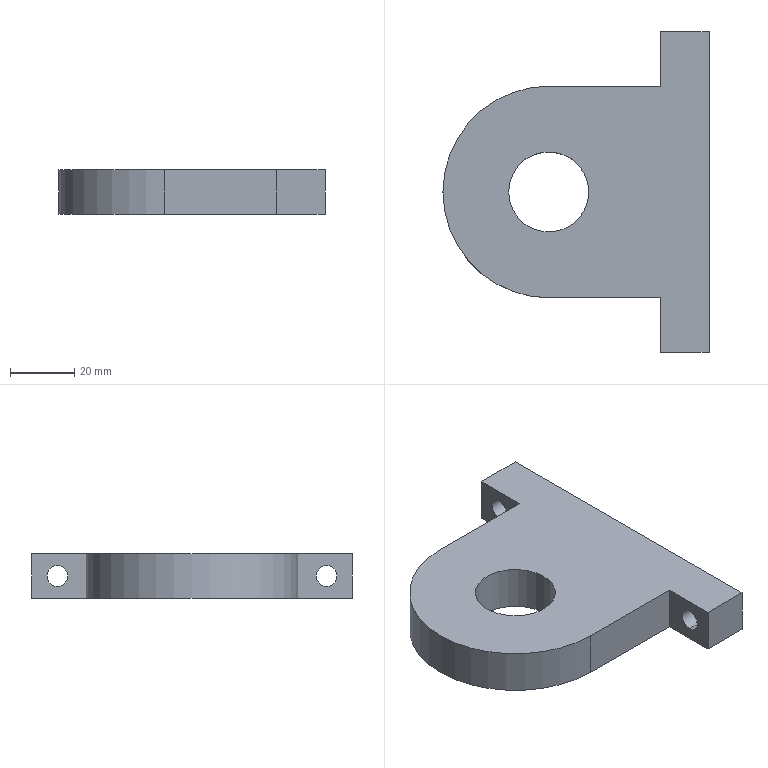Part | Creo | features DATUM PLANE 3, CURVE 2, COORDINATE SYSTEM 1, CUT 1, PROTRUSION 1 | 1 solid | 16 faces | box 83 x 100 x 14 mm | volume 69421 mm3 | plane 9 | cylinder 7 | commonest cylinder face diameters 6.5 x4 25 x2 66 x1
STEP:
#1=CARTESIAN_POINT('',(0.,0.,0.));
#2=DIRECTION('',(0.,0.,1.));
#3=DIRECTION('',(1.,0.,0.));
#4=AXIS2_PLACEMENT_3D('',#1,#2,#3);
#5=CARTESIAN_POINT('',(50.,50.,0.));
#6=VERTEX_POINT('',#5);
#7=CARTESIAN_POINT('',(35.,50.,0.));
#8=VERTEX_POINT('',#7);
#9=CARTESIAN_POINT('',(50.,50.,0.));
#10=DIRECTION('',(-1.,0.,0.));
#11=VECTOR('',#10,15.);
#12=LINE('',#9,#11);
#13=EDGE_CURVE('',#6,#8,#12,.T.);
#14=ORIENTED_EDGE('',*,*,#13,.T.);
#15=CARTESIAN_POINT('',(35.,33.,0.));
#16=VERTEX_POINT('',#15);
#17=CARTESIAN_POINT('',(35.,50.,0.));
#18=DIRECTION('',(0.,-1.,0.));
#19=VECTOR('',#18,17.);
#20=LINE('',#17,#19);
#21=EDGE_CURVE('',#8,#16,#20,.T.);
#22=ORIENTED_EDGE('',*,*,#21,.T.);
#23=CARTESIAN_POINT('',(0.,33.,0.));
#24=VERTEX_POINT('',#23);
#25=CARTESIAN_POINT('',(35.,33.,0.));
#26=DIRECTION('',(-1.,0.,0.));
#27=VECTOR('',#26,35.);
#28=LINE('',#25,#27);
#29=EDGE_CURVE('',#16,#24,#28,.T.);
#30=ORIENTED_EDGE('',*,*,#29,.T.);
#31=CARTESIAN_POINT('',(0.,-33.,0.));
#32=VERTEX_POINT('',#31);
#33=CARTESIAN_POINT('',(0.,0.,0.));
#34=DIRECTION('',(0.,0.,1.));
#35=DIRECTION('',(0.,1.,0.));
#36=AXIS2_PLACEMENT_3D('',#33,#34,#35);
#37=CIRCLE('',#36,33.);
#38=EDGE_CURVE('',#24,#32,#37,.T.);
#39=ORIENTED_EDGE('',*,*,#38,.T.);
#40=CARTESIAN_POINT('',(35.,-33.,0.));
#41=VERTEX_POINT('',#40);
#42=CARTESIAN_POINT('',(0.,-33.,0.));
#43=DIRECTION('',(1.,0.,0.));
#44=VECTOR('',#43,35.);
#45=LINE('',#42,#44);
#46=EDGE_CURVE('',#32,#41,#45,.T.);
#47=ORIENTED_EDGE('',*,*,#46,.T.);
#48=CARTESIAN_POINT('',(35.,-50.,0.));
#49=VERTEX_POINT('',#48);
#50=CARTESIAN_POINT('',(35.,-33.,0.));
#51=DIRECTION('',(0.,-1.,0.));
#52=VECTOR('',#51,17.);
#53=LINE('',#50,#52);
#54=EDGE_CURVE('',#41,#49,#53,.T.);
#55=ORIENTED_EDGE('',*,*,#54,.T.);
#56=CARTESIAN_POINT('',(50.,-50.,0.));
#57=VERTEX_POINT('',#56);
#58=CARTESIAN_POINT('',(35.,-50.,0.));
#59=DIRECTION('',(1.,0.,0.));
#60=VECTOR('',#59,15.);
#61=LINE('',#58,#60);
#62=EDGE_CURVE('',#49,#57,#61,.T.);
#63=ORIENTED_EDGE('',*,*,#62,.T.);
#64=CARTESIAN_POINT('',(50.,-50.,0.));
#65=DIRECTION('',(0.,1.,0.));
#66=VECTOR('',#65,100.);
#67=LINE('',#64,#66);
#68=EDGE_CURVE('',#57,#6,#67,.T.);
#69=ORIENTED_EDGE('',*,*,#68,.T.);
#70=EDGE_LOOP('',(#14,#22,#30,#39,#47,#55,#63,#69));
#71=FACE_OUTER_BOUND('',#70,.F.);
#72=CARTESIAN_POINT('',(12.5,0.,0.));
#73=VERTEX_POINT('',#72);
#74=CARTESIAN_POINT('',(-12.5,0.,0.));
#75=VERTEX_POINT('',#74);
#76=CARTESIAN_POINT('',(0.,0.,0.));
#77=DIRECTION('',(0.,0.,-1.));
#78=DIRECTION('',(1.,0.,0.));
#79=AXIS2_PLACEMENT_3D('',#76,#77,#78);
#80=CIRCLE('',#79,12.5);
#81=EDGE_CURVE('',#73,#75,#80,.T.);
#82=ORIENTED_EDGE('',*,*,#81,.T.);
#83=CARTESIAN_POINT('',(0.,0.,0.));
#84=DIRECTION('',(0.,0.,-1.));
#85=DIRECTION('',(-1.,0.,0.));
#86=AXIS2_PLACEMENT_3D('',#83,#84,#85);
#87=CIRCLE('',#86,12.5);
#88=EDGE_CURVE('',#75,#73,#87,.T.);
#89=ORIENTED_EDGE('',*,*,#88,.T.);
#90=EDGE_LOOP('',(#82,#89));
#91=FACE_BOUND('',#90,.F.);
#92=CARTESIAN_POINT('',(0.,0.,0.));
#93=DIRECTION('',(0.,0.,1.));
#94=DIRECTION('',(1.,0.,0.));
#95=AXIS2_PLACEMENT_3D('',#92,#93,#94);
#96=PLANE('',#95);
#97=ADVANCED_FACE('',(#71,#91),#96,.F.);
#98=ORIENTED_EDGE('',*,*,#81,.F.);
#99=CARTESIAN_POINT('',(12.5,0.,14.));
#100=VERTEX_POINT('',#99);
#101=CARTESIAN_POINT('',(12.5,0.,0.));
#102=DIRECTION('',(0.,0.,1.));
#103=VECTOR('',#102,14.);
#104=LINE('',#101,#103);
#105=EDGE_CURVE('',#73,#100,#104,.T.);
#106=ORIENTED_EDGE('',*,*,#105,.T.);
#107=CARTESIAN_POINT('',(-12.5,0.,14.));
#108=VERTEX_POINT('',#107);
#109=CARTESIAN_POINT('',(0.,0.,14.));
#110=DIRECTION('',(0.,0.,-1.));
#111=DIRECTION('',(1.,0.,0.));
#112=AXIS2_PLACEMENT_3D('',#109,#110,#111);
#113=CIRCLE('',#112,12.5);
#114=EDGE_CURVE('',#100,#108,#113,.T.);
#115=ORIENTED_EDGE('',*,*,#114,.T.);
#116=CARTESIAN_POINT('',(-12.5,0.,0.));
#117=DIRECTION('',(0.,0.,1.));
#118=VECTOR('',#117,14.);
#119=LINE('',#116,#118);
#120=EDGE_CURVE('',#75,#108,#119,.T.);
#121=ORIENTED_EDGE('',*,*,#120,.F.);
#122=EDGE_LOOP('',(#98,#106,#115,#121));
#123=FACE_OUTER_BOUND('',#122,.F.);
#124=CARTESIAN_POINT('',(0.,0.,0.));
#125=DIRECTION('',(0.,0.,1.));
#126=DIRECTION('',(1.,0.,0.));
#127=AXIS2_PLACEMENT_3D('',#124,#125,#126);
#128=CYLINDRICAL_SURFACE('',#127,12.5);
#129=ADVANCED_FACE('',(#123),#128,.F.);
#130=ORIENTED_EDGE('',*,*,#88,.F.);
#131=ORIENTED_EDGE('',*,*,#120,.T.);
#132=CARTESIAN_POINT('',(0.,0.,14.));
#133=DIRECTION('',(0.,0.,-1.));
#134=DIRECTION('',(-1.,0.,0.));
#135=AXIS2_PLACEMENT_3D('',#132,#133,#134);
#136=CIRCLE('',#135,12.5);
#137=EDGE_CURVE('',#108,#100,#136,.T.);
#138=ORIENTED_EDGE('',*,*,#137,.T.);
#139=ORIENTED_EDGE('',*,*,#105,.F.);
#140=EDGE_LOOP('',(#130,#131,#138,#139));
#141=FACE_OUTER_BOUND('',#140,.F.);
#142=CARTESIAN_POINT('',(0.,0.,0.));
#143=DIRECTION('',(0.,0.,1.));
#144=DIRECTION('',(1.,0.,0.));
#145=AXIS2_PLACEMENT_3D('',#142,#143,#144);
#146=CYLINDRICAL_SURFACE('',#145,12.5);
#147=ADVANCED_FACE('',(#141),#146,.F.);
#148=CARTESIAN_POINT('',(50.,50.,14.));
#149=VERTEX_POINT('',#148);
#150=CARTESIAN_POINT('',(35.,50.,14.));
#151=VERTEX_POINT('',#150);
#152=CARTESIAN_POINT('',(50.,50.,14.));
#153=DIRECTION('',(-1.,0.,0.));
#154=VECTOR('',#153,15.);
#155=LINE('',#152,#154);
#156=EDGE_CURVE('',#149,#151,#155,.T.);
#157=ORIENTED_EDGE('',*,*,#156,.F.);
#158=CARTESIAN_POINT('',(50.,-50.,14.));
#159=VERTEX_POINT('',#158);
#160=CARTESIAN_POINT('',(50.,-50.,14.));
#161=DIRECTION('',(0.,1.,0.));
#162=VECTOR('',#161,100.);
#163=LINE('',#160,#162);
#164=EDGE_CURVE('',#159,#149,#163,.T.);
#165=ORIENTED_EDGE('',*,*,#164,.F.);
#166=CARTESIAN_POINT('',(35.,-50.,14.));
#167=VERTEX_POINT('',#166);
#168=CARTESIAN_POINT('',(35.,-50.,14.));
#169=DIRECTION('',(1.,0.,0.));
#170=VECTOR('',#169,15.);
#171=LINE('',#168,#170);
#172=EDGE_CURVE('',#167,#159,#171,.T.);
#173=ORIENTED_EDGE('',*,*,#172,.F.);
#174=CARTESIAN_POINT('',(35.,-33.,14.));
#175=VERTEX_POINT('',#174);
#176=CARTESIAN_POINT('',(35.,-33.,14.));
#177=DIRECTION('',(0.,-1.,0.));
#178=VECTOR('',#177,17.);
#179=LINE('',#176,#178);
#180=EDGE_CURVE('',#175,#167,#179,.T.);
#181=ORIENTED_EDGE('',*,*,#180,.F.);
#182=CARTESIAN_POINT('',(0.,-33.,14.));
#183=VERTEX_POINT('',#182);
#184=CARTESIAN_POINT('',(0.,-33.,14.));
#185=DIRECTION('',(1.,0.,0.));
#186=VECTOR('',#185,35.);
#187=LINE('',#184,#186);
#188=EDGE_CURVE('',#183,#175,#187,.T.);
#189=ORIENTED_EDGE('',*,*,#188,.F.);
#190=CARTESIAN_POINT('',(0.,33.,14.));
#191=VERTEX_POINT('',#190);
#192=CARTESIAN_POINT('',(0.,0.,14.));
#193=DIRECTION('',(0.,0.,1.));
#194=DIRECTION('',(0.,1.,0.));
#195=AXIS2_PLACEMENT_3D('',#192,#193,#194);
#196=CIRCLE('',#195,33.);
#197=EDGE_CURVE('',#191,#183,#196,.T.);
#198=ORIENTED_EDGE('',*,*,#197,.F.);
#199=CARTESIAN_POINT('',(35.,33.,14.));
#200=VERTEX_POINT('',#199);
#201=CARTESIAN_POINT('',(35.,33.,14.));
#202=DIRECTION('',(-1.,0.,0.));
#203=VECTOR('',#202,35.);
#204=LINE('',#201,#203);
#205=EDGE_CURVE('',#200,#191,#204,.T.);
#206=ORIENTED_EDGE('',*,*,#205,.F.);
#207=CARTESIAN_POINT('',(35.,50.,14.));
#208=DIRECTION('',(0.,-1.,0.));
#209=VECTOR('',#208,17.);
#210=LINE('',#207,#209);
#211=EDGE_CURVE('',#151,#200,#210,.T.);
#212=ORIENTED_EDGE('',*,*,#211,.F.);
#213=EDGE_LOOP('',(#157,#165,#173,#181,#189,#198,#206,#212));
#214=FACE_OUTER_BOUND('',#213,.F.);
#215=ORIENTED_EDGE('',*,*,#114,.F.);
#216=ORIENTED_EDGE('',*,*,#137,.F.);
#217=EDGE_LOOP('',(#215,#216));
#218=FACE_BOUND('',#217,.F.);
#219=CARTESIAN_POINT('',(0.,0.,14.));
#220=DIRECTION('',(0.,0.,1.));
#221=DIRECTION('',(1.,0.,0.));
#222=AXIS2_PLACEMENT_3D('',#219,#220,#221);
#223=PLANE('',#222);
#224=ADVANCED_FACE('',(#214,#218),#223,.T.);
#225=ORIENTED_EDGE('',*,*,#13,.F.);
#226=CARTESIAN_POINT('',(50.,50.,0.));
#227=DIRECTION('',(0.,0.,1.));
#228=VECTOR('',#227,14.);
#229=LINE('',#226,#228);
#230=EDGE_CURVE('',#6,#149,#229,.T.);
#231=ORIENTED_EDGE('',*,*,#230,.T.);
#232=ORIENTED_EDGE('',*,*,#156,.T.);
#233=CARTESIAN_POINT('',(35.,50.,0.));
#234=DIRECTION('',(0.,0.,1.));
#235=VECTOR('',#234,14.);
#236=LINE('',#233,#235);
#237=EDGE_CURVE('',#8,#151,#236,.T.);
#238=ORIENTED_EDGE('',*,*,#237,.F.);
#239=EDGE_LOOP('',(#225,#231,#232,#238));
#240=FACE_OUTER_BOUND('',#239,.F.);
#241=CARTESIAN_POINT('',(50.,50.,0.));
#242=DIRECTION('',(0.,1.,0.));
#243=DIRECTION('',(-1.,0.,0.));
#244=AXIS2_PLACEMENT_3D('',#241,#242,#243);
#245=PLANE('',#244);
#246=ADVANCED_FACE('',(#240),#245,.T.);
#247=ORIENTED_EDGE('',*,*,#68,.F.);
#248=CARTESIAN_POINT('',(50.,-50.,0.));
#249=DIRECTION('',(0.,0.,1.));
#250=VECTOR('',#249,14.);
#251=LINE('',#248,#250);
#252=EDGE_CURVE('',#57,#159,#251,.T.);
#253=ORIENTED_EDGE('',*,*,#252,.T.);
#254=ORIENTED_EDGE('',*,*,#164,.T.);
#255=ORIENTED_EDGE('',*,*,#230,.F.);
#256=EDGE_LOOP('',(#247,#253,#254,#255));
#257=FACE_OUTER_BOUND('',#256,.F.);
#258=CARTESIAN_POINT('',(50.,42.,10.25));
#259=VERTEX_POINT('',#258);
#260=CARTESIAN_POINT('',(50.,42.,3.75));
#261=VERTEX_POINT('',#260);
#262=CARTESIAN_POINT('',(50.,42.,7.));
#263=DIRECTION('',(-1.,0.,0.));
#264=DIRECTION('',(0.,0.,1.));
#265=AXIS2_PLACEMENT_3D('',#262,#263,#264);
#266=CIRCLE('',#265,3.25);
#267=EDGE_CURVE('',#259,#261,#266,.T.);
#268=ORIENTED_EDGE('',*,*,#267,.F.);
#269=CARTESIAN_POINT('',(50.,42.,7.));
#270=DIRECTION('',(-1.,0.,0.));
#271=DIRECTION('',(0.,0.,-1.));
#272=AXIS2_PLACEMENT_3D('',#269,#270,#271);
#273=CIRCLE('',#272,3.25);
#274=EDGE_CURVE('',#261,#259,#273,.T.);
#275=ORIENTED_EDGE('',*,*,#274,.F.);
#276=EDGE_LOOP('',(#268,#275));
#277=FACE_BOUND('',#276,.F.);
#278=CARTESIAN_POINT('',(50.,-42.,10.25));
#279=VERTEX_POINT('',#278);
#280=CARTESIAN_POINT('',(50.,-42.,3.75));
#281=VERTEX_POINT('',#280);
#282=CARTESIAN_POINT('',(50.,-42.,7.));
#283=DIRECTION('',(-1.,0.,0.));
#284=DIRECTION('',(0.,0.,1.));
#285=AXIS2_PLACEMENT_3D('',#282,#283,#284);
#286=CIRCLE('',#285,3.25);
#287=EDGE_CURVE('',#279,#281,#286,.T.);
#288=ORIENTED_EDGE('',*,*,#287,.F.);
#289=CARTESIAN_POINT('',(50.,-42.,7.));
#290=DIRECTION('',(-1.,0.,0.));
#291=DIRECTION('',(0.,0.,-1.));
#292=AXIS2_PLACEMENT_3D('',#289,#290,#291);
#293=CIRCLE('',#292,3.25);
#294=EDGE_CURVE('',#281,#279,#293,.T.);
#295=ORIENTED_EDGE('',*,*,#294,.F.);
#296=EDGE_LOOP('',(#288,#295));
#297=FACE_BOUND('',#296,.F.);
#298=CARTESIAN_POINT('',(50.,-50.,0.));
#299=DIRECTION('',(1.,0.,0.));
#300=DIRECTION('',(0.,1.,0.));
#301=AXIS2_PLACEMENT_3D('',#298,#299,#300);
#302=PLANE('',#301);
#303=ADVANCED_FACE('',(#257,#277,#297),#302,.T.);
#304=ORIENTED_EDGE('',*,*,#62,.F.);
#305=CARTESIAN_POINT('',(35.,-50.,0.));
#306=DIRECTION('',(0.,0.,1.));
#307=VECTOR('',#306,14.);
#308=LINE('',#305,#307);
#309=EDGE_CURVE('',#49,#167,#308,.T.);
#310=ORIENTED_EDGE('',*,*,#309,.T.);
#311=ORIENTED_EDGE('',*,*,#172,.T.);
#312=ORIENTED_EDGE('',*,*,#252,.F.);
#313=EDGE_LOOP('',(#304,#310,#311,#312));
#314=FACE_OUTER_BOUND('',#313,.F.);
#315=CARTESIAN_POINT('',(35.,-50.,0.));
#316=DIRECTION('',(0.,-1.,0.));
#317=DIRECTION('',(1.,0.,0.));
#318=AXIS2_PLACEMENT_3D('',#315,#316,#317);
#319=PLANE('',#318);
#320=ADVANCED_FACE('',(#314),#319,.T.);
#321=ORIENTED_EDGE('',*,*,#54,.F.);
#322=CARTESIAN_POINT('',(35.,-33.,0.));
#323=DIRECTION('',(0.,0.,1.));
#324=VECTOR('',#323,14.);
#325=LINE('',#322,#324);
#326=EDGE_CURVE('',#41,#175,#325,.T.);
#327=ORIENTED_EDGE('',*,*,#326,.T.);
#328=ORIENTED_EDGE('',*,*,#180,.T.);
#329=ORIENTED_EDGE('',*,*,#309,.F.);
#330=EDGE_LOOP('',(#321,#327,#328,#329));
#331=FACE_OUTER_BOUND('',#330,.F.);
#332=CARTESIAN_POINT('',(35.,-42.,10.25));
#333=VERTEX_POINT('',#332);
#334=CARTESIAN_POINT('',(35.,-42.,3.75));
#335=VERTEX_POINT('',#334);
#336=CARTESIAN_POINT('',(35.,-42.,7.));
#337=DIRECTION('',(-1.,0.,0.));
#338=DIRECTION('',(0.,0.,1.));
#339=AXIS2_PLACEMENT_3D('',#336,#337,#338);
#340=CIRCLE('',#339,3.25);
#341=EDGE_CURVE('',#333,#335,#340,.T.);
#342=ORIENTED_EDGE('',*,*,#341,.T.);
#343=CARTESIAN_POINT('',(35.,-42.,7.));
#344=DIRECTION('',(-1.,0.,0.));
#345=DIRECTION('',(0.,0.,-1.));
#346=AXIS2_PLACEMENT_3D('',#343,#344,#345);
#347=CIRCLE('',#346,3.25);
#348=EDGE_CURVE('',#335,#333,#347,.T.);
#349=ORIENTED_EDGE('',*,*,#348,.T.);
#350=EDGE_LOOP('',(#342,#349));
#351=FACE_BOUND('',#350,.F.);
#352=CARTESIAN_POINT('',(35.,-33.,0.));
#353=DIRECTION('',(-1.,0.,0.));
#354=DIRECTION('',(0.,-1.,0.));
#355=AXIS2_PLACEMENT_3D('',#352,#353,#354);
#356=PLANE('',#355);
#357=ADVANCED_FACE('',(#331,#351),#356,.T.);
#358=ORIENTED_EDGE('',*,*,#46,.F.);
#359=CARTESIAN_POINT('',(0.,-33.,0.));
#360=DIRECTION('',(0.,0.,1.));
#361=VECTOR('',#360,14.);
#362=LINE('',#359,#361);
#363=EDGE_CURVE('',#32,#183,#362,.T.);
#364=ORIENTED_EDGE('',*,*,#363,.T.);
#365=ORIENTED_EDGE('',*,*,#188,.T.);
#366=ORIENTED_EDGE('',*,*,#326,.F.);
#367=EDGE_LOOP('',(#358,#364,#365,#366));
#368=FACE_OUTER_BOUND('',#367,.F.);
#369=CARTESIAN_POINT('',(0.,-33.,0.));
#370=DIRECTION('',(0.,-1.,0.));
#371=DIRECTION('',(1.,0.,0.));
#372=AXIS2_PLACEMENT_3D('',#369,#370,#371);
#373=PLANE('',#372);
#374=ADVANCED_FACE('',(#368),#373,.T.);
#375=ORIENTED_EDGE('',*,*,#38,.F.);
#376=CARTESIAN_POINT('',(0.,33.,0.));
#377=DIRECTION('',(0.,0.,1.));
#378=VECTOR('',#377,14.);
#379=LINE('',#376,#378);
#380=EDGE_CURVE('',#24,#191,#379,.T.);
#381=ORIENTED_EDGE('',*,*,#380,.T.);
#382=ORIENTED_EDGE('',*,*,#197,.T.);
#383=ORIENTED_EDGE('',*,*,#363,.F.);
#384=EDGE_LOOP('',(#375,#381,#382,#383));
#385=FACE_OUTER_BOUND('',#384,.F.);
#386=CARTESIAN_POINT('',(0.,0.,0.));
#387=DIRECTION('',(0.,0.,1.));
#388=DIRECTION('',(1.,0.,0.));
#389=AXIS2_PLACEMENT_3D('',#386,#387,#388);
#390=CYLINDRICAL_SURFACE('',#389,33.);
#391=ADVANCED_FACE('',(#385),#390,.T.);
#392=ORIENTED_EDGE('',*,*,#29,.F.);
#393=CARTESIAN_POINT('',(35.,33.,0.));
#394=DIRECTION('',(0.,0.,1.));
#395=VECTOR('',#394,14.);
#396=LINE('',#393,#395);
#397=EDGE_CURVE('',#16,#200,#396,.T.);
#398=ORIENTED_EDGE('',*,*,#397,.T.);
#399=ORIENTED_EDGE('',*,*,#205,.T.);
#400=ORIENTED_EDGE('',*,*,#380,.F.);
#401=EDGE_LOOP('',(#392,#398,#399,#400));
#402=FACE_OUTER_BOUND('',#401,.F.);
#403=CARTESIAN_POINT('',(35.,33.,0.));
#404=DIRECTION('',(0.,1.,0.));
#405=DIRECTION('',(-1.,0.,0.));
#406=AXIS2_PLACEMENT_3D('',#403,#404,#405);
#407=PLANE('',#406);
#408=ADVANCED_FACE('',(#402),#407,.T.);
#409=ORIENTED_EDGE('',*,*,#21,.F.);
#410=ORIENTED_EDGE('',*,*,#237,.T.);
#411=ORIENTED_EDGE('',*,*,#211,.T.);
#412=ORIENTED_EDGE('',*,*,#397,.F.);
#413=EDGE_LOOP('',(#409,#410,#411,#412));
#414=FACE_OUTER_BOUND('',#413,.F.);
#415=CARTESIAN_POINT('',(35.,42.,10.25));
#416=VERTEX_POINT('',#415);
#417=CARTESIAN_POINT('',(35.,42.,3.75));
#418=VERTEX_POINT('',#417);
#419=CARTESIAN_POINT('',(35.,42.,7.));
#420=DIRECTION('',(-1.,0.,0.));
#421=DIRECTION('',(0.,0.,1.));
#422=AXIS2_PLACEMENT_3D('',#419,#420,#421);
#423=CIRCLE('',#422,3.25);
#424=EDGE_CURVE('',#416,#418,#423,.T.);
#425=ORIENTED_EDGE('',*,*,#424,.T.);
#426=CARTESIAN_POINT('',(35.,42.,7.));
#427=DIRECTION('',(-1.,0.,0.));
#428=DIRECTION('',(0.,0.,-1.));
#429=AXIS2_PLACEMENT_3D('',#426,#427,#428);
#430=CIRCLE('',#429,3.25);
#431=EDGE_CURVE('',#418,#416,#430,.T.);
#432=ORIENTED_EDGE('',*,*,#431,.T.);
#433=EDGE_LOOP('',(#425,#432));
#434=FACE_BOUND('',#433,.F.);
#435=CARTESIAN_POINT('',(35.,50.,0.));
#436=DIRECTION('',(-1.,0.,0.));
#437=DIRECTION('',(0.,-1.,0.));
#438=AXIS2_PLACEMENT_3D('',#435,#436,#437);
#439=PLANE('',#438);
#440=ADVANCED_FACE('',(#414,#434),#439,.T.);
#441=ORIENTED_EDGE('',*,*,#424,.F.);
#442=CARTESIAN_POINT('',(35.,42.,10.25));
#443=DIRECTION('',(1.,0.,0.));
#444=VECTOR('',#443,15.);
#445=LINE('',#442,#444);
#446=EDGE_CURVE('',#416,#259,#445,.T.);
#447=ORIENTED_EDGE('',*,*,#446,.T.);
#448=ORIENTED_EDGE('',*,*,#267,.T.);
#449=CARTESIAN_POINT('',(35.,42.,3.75));
#450=DIRECTION('',(1.,0.,0.));
#451=VECTOR('',#450,15.);
#452=LINE('',#449,#451);
#453=EDGE_CURVE('',#418,#261,#452,.T.);
#454=ORIENTED_EDGE('',*,*,#453,.F.);
#455=EDGE_LOOP('',(#441,#447,#448,#454));
#456=FACE_OUTER_BOUND('',#455,.F.);
#457=CARTESIAN_POINT('',(35.,42.,7.));
#458=DIRECTION('',(-1.,0.,0.));
#459=DIRECTION('',(0.,0.,1.));
#460=AXIS2_PLACEMENT_3D('',#457,#458,#459);
#461=CYLINDRICAL_SURFACE('',#460,3.25);
#462=ADVANCED_FACE('',(#456),#461,.F.);
#463=ORIENTED_EDGE('',*,*,#431,.F.);
#464=ORIENTED_EDGE('',*,*,#453,.T.);
#465=ORIENTED_EDGE('',*,*,#274,.T.);
#466=ORIENTED_EDGE('',*,*,#446,.F.);
#467=EDGE_LOOP('',(#463,#464,#465,#466));
#468=FACE_OUTER_BOUND('',#467,.F.);
#469=CARTESIAN_POINT('',(35.,42.,7.));
#470=DIRECTION('',(-1.,0.,0.));
#471=DIRECTION('',(0.,0.,1.));
#472=AXIS2_PLACEMENT_3D('',#469,#470,#471);
#473=CYLINDRICAL_SURFACE('',#472,3.25);
#474=ADVANCED_FACE('',(#468),#473,.F.);
#475=ORIENTED_EDGE('',*,*,#341,.F.);
#476=CARTESIAN_POINT('',(35.,-42.,10.25));
#477=DIRECTION('',(1.,0.,0.));
#478=VECTOR('',#477,15.);
#479=LINE('',#476,#478);
#480=EDGE_CURVE('',#333,#279,#479,.T.);
#481=ORIENTED_EDGE('',*,*,#480,.T.);
#482=ORIENTED_EDGE('',*,*,#287,.T.);
#483=CARTESIAN_POINT('',(35.,-42.,3.75));
#484=DIRECTION('',(1.,0.,0.));
#485=VECTOR('',#484,15.);
#486=LINE('',#483,#485);
#487=EDGE_CURVE('',#335,#281,#486,.T.);
#488=ORIENTED_EDGE('',*,*,#487,.F.);
#489=EDGE_LOOP('',(#475,#481,#482,#488));
#490=FACE_OUTER_BOUND('',#489,.F.);
#491=CARTESIAN_POINT('',(35.,-42.,7.));
#492=DIRECTION('',(-1.,0.,0.));
#493=DIRECTION('',(0.,0.,1.));
#494=AXIS2_PLACEMENT_3D('',#491,#492,#493);
#495=CYLINDRICAL_SURFACE('',#494,3.25);
#496=ADVANCED_FACE('',(#490),#495,.F.);
#497=ORIENTED_EDGE('',*,*,#348,.F.);
#498=ORIENTED_EDGE('',*,*,#487,.T.);
#499=ORIENTED_EDGE('',*,*,#294,.T.);
#500=ORIENTED_EDGE('',*,*,#480,.F.);
#501=EDGE_LOOP('',(#497,#498,#499,#500));
#502=FACE_OUTER_BOUND('',#501,.F.);
#503=CARTESIAN_POINT('',(35.,-42.,7.));
#504=DIRECTION('',(-1.,0.,0.));
#505=DIRECTION('',(0.,0.,1.));
#506=AXIS2_PLACEMENT_3D('',#503,#504,#505);
#507=CYLINDRICAL_SURFACE('',#506,3.25);
#508=ADVANCED_FACE('',(#502),#507,.F.);
#509=CLOSED_SHELL('',(#97,#129,#147,#224,#246,#303,#320,#357,#374,#391,#408,#440,#462,#474,#496,#508));
#510=MANIFOLD_SOLID_BREP('',#509);
#511=(LENGTH_UNIT()NAMED_UNIT(*)SI_UNIT(.MILLI.,.METRE.));
#512=UNCERTAINTY_MEASURE_WITH_UNIT(LENGTH_MEASURE(0.01307),#511,'','');
#513=(NAMED_UNIT(*)PLANE_ANGLE_UNIT()SI_UNIT($,.RADIAN.));
#514=PLANE_ANGLE_MEASURE_WITH_UNIT(PLANE_ANGLE_MEASURE(0.01745),#513);
#515=(CONVERSION_BASED_UNIT('DEGREE',#514)NAMED_UNIT(*)PLANE_ANGLE_UNIT());
#516=(NAMED_UNIT(*)SI_UNIT($,.STERADIAN.)SOLID_ANGLE_UNIT());
#517=(GEOMETRIC_REPRESENTATION_CONTEXT(3)GLOBAL_UNCERTAINTY_ASSIGNED_CONTEXT((#512))GLOBAL_UNIT_ASSIGNED_CONTEXT((#511,#515,#516))REPRESENTATION_CONTEXT('',''));
#518=ADVANCED_BREP_SHAPE_REPRESENTATION('',(#4,#510),#517);